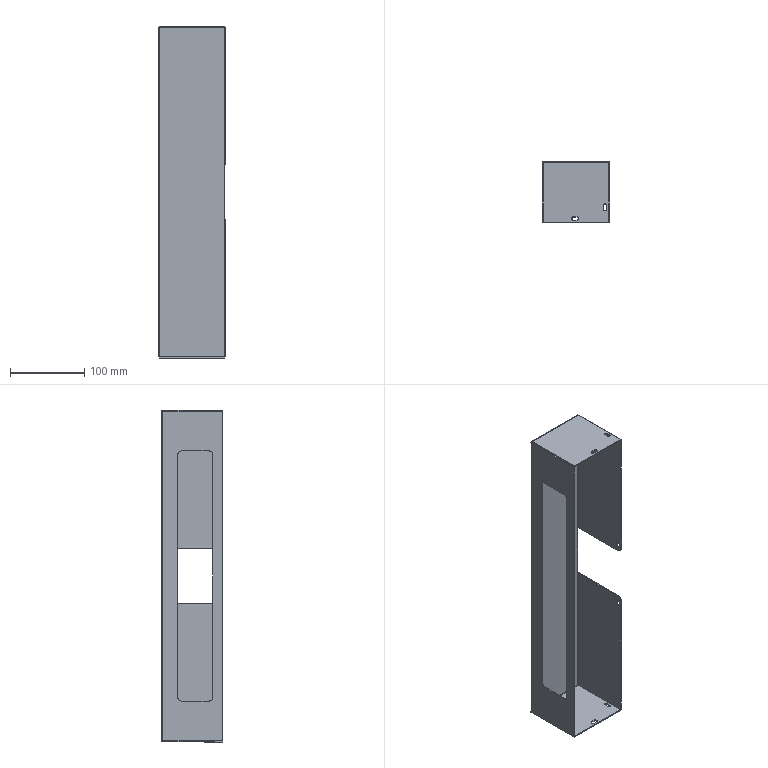Part | SolidWorks | features Cut 4, EdgeFlange 1, Fillet 1, FlatPattern 1, SMBaseFlange 1, SheetMetal 1 | 1 solid | 86 faces | box 91 x 82 x 446 mm | volume 155012 mm3 | plane 56 | cylinder 30 | commonest cylinder face diameters 4.5 x14 10 x6 0.6 x5 3.6 x5